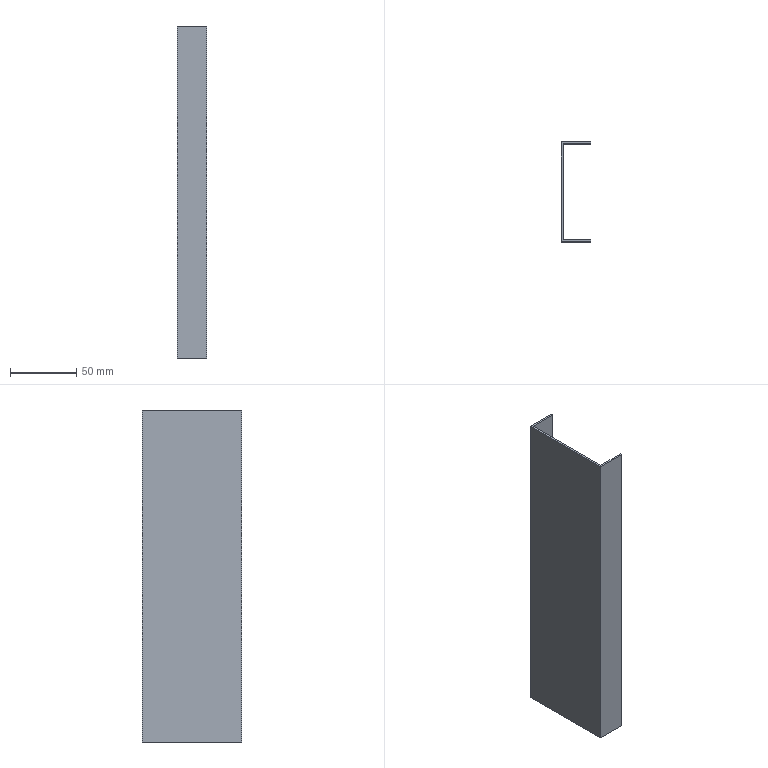Part | STEP file | Guide wheel mechanism revised.sldasm-Part-186 | 1 solid | 10 faces | box 22.5 x 75 x 250 mm | volume 43875 mm3 | plane 10
STEP:
#1=CARTESIAN_POINT('',(337.5,655.,202.));
#2=VERTEX_POINT('',#1);
#3=CARTESIAN_POINT('',(360.,655.,202.));
#4=VERTEX_POINT('',#3);
#5=CARTESIAN_POINT('',(337.5,655.,202.));
#6=DIRECTION('',(1.,0.,0.));
#7=VECTOR('',#6,1000.);
#8=LINE('',#5,#7);
#9=EDGE_CURVE('',#2,#4,#8,.T.);
#10=ORIENTED_EDGE('',*,*,#9,.F.);
#11=CARTESIAN_POINT('',(337.5,655.,-48.));
#12=VERTEX_POINT('',#11);
#13=CARTESIAN_POINT('',(337.5,655.,-48.));
#14=DIRECTION('',(0.,0.,1.));
#15=VECTOR('',#14,1000.);
#16=LINE('',#13,#15);
#17=EDGE_CURVE('',#12,#2,#16,.T.);
#18=ORIENTED_EDGE('',*,*,#17,.F.);
#19=CARTESIAN_POINT('',(360.,655.,-48.));
#20=VERTEX_POINT('',#19);
#21=CARTESIAN_POINT('',(337.5,655.,-48.));
#22=DIRECTION('',(1.,0.,0.));
#23=VECTOR('',#22,1000.);
#24=LINE('',#21,#23);
#25=EDGE_CURVE('',#12,#20,#24,.T.);
#26=ORIENTED_EDGE('',*,*,#25,.T.);
#27=CARTESIAN_POINT('',(360.,655.,-48.));
#28=DIRECTION('',(0.,0.,1.));
#29=VECTOR('',#28,1000.);
#30=LINE('',#27,#29);
#31=EDGE_CURVE('',#20,#4,#30,.T.);
#32=ORIENTED_EDGE('',*,*,#31,.T.);
#33=EDGE_LOOP('',(#10,#18,#26,#32));
#34=FACE_OUTER_BOUND('',#33,.T.);
#35=CARTESIAN_POINT('',(337.5,655.,-48.));
#36=DIRECTION('',(0.,-1.,0.));
#37=DIRECTION('',(0.,0.,-1.));
#38=AXIS2_PLACEMENT_3D('',#35,#36,#37);
#39=PLANE('',#38);
#40=ADVANCED_FACE('',(#34),#39,.T.);
#41=CARTESIAN_POINT('',(337.5,730.,202.));
#42=VERTEX_POINT('',#41);
#43=CARTESIAN_POINT('',(337.5,730.,202.));
#44=DIRECTION('',(0.,-1.,0.));
#45=VECTOR('',#44,1000.);
#46=LINE('',#43,#45);
#47=EDGE_CURVE('',#42,#2,#46,.T.);
#48=ORIENTED_EDGE('',*,*,#47,.F.);
#49=CARTESIAN_POINT('',(337.5,730.,-48.));
#50=VERTEX_POINT('',#49);
#51=CARTESIAN_POINT('',(337.5,730.,-48.));
#52=DIRECTION('',(0.,0.,1.));
#53=VECTOR('',#52,1000.);
#54=LINE('',#51,#53);
#55=EDGE_CURVE('',#50,#42,#54,.T.);
#56=ORIENTED_EDGE('',*,*,#55,.F.);
#57=CARTESIAN_POINT('',(337.5,730.,-48.));
#58=DIRECTION('',(0.,-1.,0.));
#59=VECTOR('',#58,1000.);
#60=LINE('',#57,#59);
#61=EDGE_CURVE('',#50,#12,#60,.T.);
#62=ORIENTED_EDGE('',*,*,#61,.T.);
#63=ORIENTED_EDGE('',*,*,#17,.T.);
#64=EDGE_LOOP('',(#48,#56,#62,#63));
#65=FACE_OUTER_BOUND('',#64,.T.);
#66=CARTESIAN_POINT('',(337.5,730.,-48.));
#67=DIRECTION('',(-1.,0.,0.));
#68=DIRECTION('',(0.,-1.,0.));
#69=AXIS2_PLACEMENT_3D('',#66,#67,#68);
#70=PLANE('',#69);
#71=ADVANCED_FACE('',(#65),#70,.T.);
#72=CARTESIAN_POINT('',(360.,730.,202.));
#73=VERTEX_POINT('',#72);
#74=CARTESIAN_POINT('',(337.5,730.,202.));
#75=DIRECTION('',(-1.,0.,0.));
#76=VECTOR('',#75,1000.);
#77=LINE('',#74,#76);
#78=EDGE_CURVE('',#73,#42,#77,.T.);
#79=ORIENTED_EDGE('',*,*,#78,.F.);
#80=CARTESIAN_POINT('',(360.,730.,-48.));
#81=VERTEX_POINT('',#80);
#82=CARTESIAN_POINT('',(360.,730.,-48.));
#83=DIRECTION('',(0.,0.,1.));
#84=VECTOR('',#83,1000.);
#85=LINE('',#82,#84);
#86=EDGE_CURVE('',#81,#73,#85,.T.);
#87=ORIENTED_EDGE('',*,*,#86,.F.);
#88=CARTESIAN_POINT('',(337.5,730.,-48.));
#89=DIRECTION('',(-1.,0.,0.));
#90=VECTOR('',#89,1000.);
#91=LINE('',#88,#90);
#92=EDGE_CURVE('',#81,#50,#91,.T.);
#93=ORIENTED_EDGE('',*,*,#92,.T.);
#94=ORIENTED_EDGE('',*,*,#55,.T.);
#95=EDGE_LOOP('',(#79,#87,#93,#94));
#96=FACE_OUTER_BOUND('',#95,.T.);
#97=CARTESIAN_POINT('',(337.5,730.,-48.));
#98=DIRECTION('',(0.,1.,0.));
#99=DIRECTION('',(0.,0.,1.));
#100=AXIS2_PLACEMENT_3D('',#97,#98,#99);
#101=PLANE('',#100);
#102=ADVANCED_FACE('',(#96),#101,.T.);
#103=CARTESIAN_POINT('',(360.,728.5,202.));
#104=VERTEX_POINT('',#103);
#105=CARTESIAN_POINT('',(360.,730.,202.));
#106=DIRECTION('',(0.,-1.,0.));
#107=VECTOR('',#106,1000.);
#108=LINE('',#105,#107);
#109=EDGE_CURVE('',#73,#104,#108,.T.);
#110=ORIENTED_EDGE('',*,*,#109,.T.);
#111=CARTESIAN_POINT('',(360.,728.5,-48.));
#112=VERTEX_POINT('',#111);
#113=CARTESIAN_POINT('',(360.,728.5,-48.));
#114=DIRECTION('',(0.,0.,1.));
#115=VECTOR('',#114,1000.);
#116=LINE('',#113,#115);
#117=EDGE_CURVE('',#112,#104,#116,.T.);
#118=ORIENTED_EDGE('',*,*,#117,.F.);
#119=CARTESIAN_POINT('',(360.,730.,-48.));
#120=DIRECTION('',(0.,-1.,0.));
#121=VECTOR('',#120,1000.);
#122=LINE('',#119,#121);
#123=EDGE_CURVE('',#81,#112,#122,.T.);
#124=ORIENTED_EDGE('',*,*,#123,.F.);
#125=ORIENTED_EDGE('',*,*,#86,.T.);
#126=EDGE_LOOP('',(#110,#118,#124,#125));
#127=FACE_OUTER_BOUND('',#126,.T.);
#128=CARTESIAN_POINT('',(360.,730.,-48.));
#129=DIRECTION('',(-1.,0.,0.));
#130=DIRECTION('',(0.,0.,1.));
#131=AXIS2_PLACEMENT_3D('',#128,#129,#130);
#132=PLANE('',#131);
#133=ADVANCED_FACE('',(#127),#132,.F.);
#134=CARTESIAN_POINT('',(339.,728.5,202.));
#135=VERTEX_POINT('',#134);
#136=CARTESIAN_POINT('',(337.5,728.5,202.));
#137=DIRECTION('',(-1.,0.,0.));
#138=VECTOR('',#137,1000.);
#139=LINE('',#136,#138);
#140=EDGE_CURVE('',#104,#135,#139,.T.);
#141=ORIENTED_EDGE('',*,*,#140,.T.);
#142=CARTESIAN_POINT('',(339.,728.5,-48.));
#143=VERTEX_POINT('',#142);
#144=CARTESIAN_POINT('',(339.,728.5,-48.));
#145=DIRECTION('',(0.,0.,1.));
#146=VECTOR('',#145,1000.);
#147=LINE('',#144,#146);
#148=EDGE_CURVE('',#143,#135,#147,.T.);
#149=ORIENTED_EDGE('',*,*,#148,.F.);
#150=CARTESIAN_POINT('',(337.5,728.5,-48.));
#151=DIRECTION('',(-1.,0.,0.));
#152=VECTOR('',#151,1000.);
#153=LINE('',#150,#152);
#154=EDGE_CURVE('',#112,#143,#153,.T.);
#155=ORIENTED_EDGE('',*,*,#154,.F.);
#156=ORIENTED_EDGE('',*,*,#117,.T.);
#157=EDGE_LOOP('',(#141,#149,#155,#156));
#158=FACE_OUTER_BOUND('',#157,.T.);
#159=CARTESIAN_POINT('',(337.5,728.5,-48.));
#160=DIRECTION('',(0.,1.,0.));
#161=DIRECTION('',(0.,0.,1.));
#162=AXIS2_PLACEMENT_3D('',#159,#160,#161);
#163=PLANE('',#162);
#164=ADVANCED_FACE('',(#158),#163,.F.);
#165=CARTESIAN_POINT('',(339.,656.5,202.));
#166=VERTEX_POINT('',#165);
#167=CARTESIAN_POINT('',(339.,730.,202.));
#168=DIRECTION('',(0.,-1.,0.));
#169=VECTOR('',#168,1000.);
#170=LINE('',#167,#169);
#171=EDGE_CURVE('',#135,#166,#170,.T.);
#172=ORIENTED_EDGE('',*,*,#171,.T.);
#173=CARTESIAN_POINT('',(339.,656.5,-48.));
#174=VERTEX_POINT('',#173);
#175=CARTESIAN_POINT('',(339.,656.5,-48.));
#176=DIRECTION('',(0.,0.,1.));
#177=VECTOR('',#176,1000.);
#178=LINE('',#175,#177);
#179=EDGE_CURVE('',#174,#166,#178,.T.);
#180=ORIENTED_EDGE('',*,*,#179,.F.);
#181=CARTESIAN_POINT('',(339.,730.,-48.));
#182=DIRECTION('',(0.,-1.,0.));
#183=VECTOR('',#182,1000.);
#184=LINE('',#181,#183);
#185=EDGE_CURVE('',#143,#174,#184,.T.);
#186=ORIENTED_EDGE('',*,*,#185,.F.);
#187=ORIENTED_EDGE('',*,*,#148,.T.);
#188=EDGE_LOOP('',(#172,#180,#186,#187));
#189=FACE_OUTER_BOUND('',#188,.T.);
#190=CARTESIAN_POINT('',(339.,730.,-48.));
#191=DIRECTION('',(-1.,0.,0.));
#192=DIRECTION('',(0.,-1.,0.));
#193=AXIS2_PLACEMENT_3D('',#190,#191,#192);
#194=PLANE('',#193);
#195=ADVANCED_FACE('',(#189),#194,.F.);
#196=CARTESIAN_POINT('',(360.,656.5,202.));
#197=VERTEX_POINT('',#196);
#198=CARTESIAN_POINT('',(337.5,656.5,202.));
#199=DIRECTION('',(1.,0.,0.));
#200=VECTOR('',#199,1000.);
#201=LINE('',#198,#200);
#202=EDGE_CURVE('',#166,#197,#201,.T.);
#203=ORIENTED_EDGE('',*,*,#202,.T.);
#204=CARTESIAN_POINT('',(360.,656.5,-48.));
#205=VERTEX_POINT('',#204);
#206=CARTESIAN_POINT('',(360.,656.5,-48.));
#207=DIRECTION('',(0.,0.,1.));
#208=VECTOR('',#207,1000.);
#209=LINE('',#206,#208);
#210=EDGE_CURVE('',#205,#197,#209,.T.);
#211=ORIENTED_EDGE('',*,*,#210,.F.);
#212=CARTESIAN_POINT('',(337.5,656.5,-48.));
#213=DIRECTION('',(1.,0.,0.));
#214=VECTOR('',#213,1000.);
#215=LINE('',#212,#214);
#216=EDGE_CURVE('',#174,#205,#215,.T.);
#217=ORIENTED_EDGE('',*,*,#216,.F.);
#218=ORIENTED_EDGE('',*,*,#179,.T.);
#219=EDGE_LOOP('',(#203,#211,#217,#218));
#220=FACE_OUTER_BOUND('',#219,.T.);
#221=CARTESIAN_POINT('',(337.5,656.5,-48.));
#222=DIRECTION('',(0.,-1.,0.));
#223=DIRECTION('',(0.,0.,-1.));
#224=AXIS2_PLACEMENT_3D('',#221,#222,#223);
#225=PLANE('',#224);
#226=ADVANCED_FACE('',(#220),#225,.F.);
#227=CARTESIAN_POINT('',(360.,656.5,202.));
#228=DIRECTION('',(0.,-1.,0.));
#229=VECTOR('',#228,1000.);
#230=LINE('',#227,#229);
#231=EDGE_CURVE('',#197,#4,#230,.T.);
#232=ORIENTED_EDGE('',*,*,#231,.T.);
#233=ORIENTED_EDGE('',*,*,#31,.F.);
#234=CARTESIAN_POINT('',(360.,656.5,-48.));
#235=DIRECTION('',(0.,-1.,0.));
#236=VECTOR('',#235,1000.);
#237=LINE('',#234,#236);
#238=EDGE_CURVE('',#205,#20,#237,.T.);
#239=ORIENTED_EDGE('',*,*,#238,.F.);
#240=ORIENTED_EDGE('',*,*,#210,.T.);
#241=EDGE_LOOP('',(#232,#233,#239,#240));
#242=FACE_OUTER_BOUND('',#241,.T.);
#243=CARTESIAN_POINT('',(360.,656.5,-48.));
#244=DIRECTION('',(-1.,0.,0.));
#245=DIRECTION('',(0.,0.,1.));
#246=AXIS2_PLACEMENT_3D('',#243,#244,#245);
#247=PLANE('',#246);
#248=ADVANCED_FACE('',(#242),#247,.F.);
#249=ORIENTED_EDGE('',*,*,#25,.F.);
#250=ORIENTED_EDGE('',*,*,#61,.F.);
#251=ORIENTED_EDGE('',*,*,#92,.F.);
#252=ORIENTED_EDGE('',*,*,#123,.T.);
#253=ORIENTED_EDGE('',*,*,#154,.T.);
#254=ORIENTED_EDGE('',*,*,#185,.T.);
#255=ORIENTED_EDGE('',*,*,#216,.T.);
#256=ORIENTED_EDGE('',*,*,#238,.T.);
#257=EDGE_LOOP('',(#249,#250,#251,#252,#253,#254,#255,#256));
#258=FACE_OUTER_BOUND('',#257,.T.);
#259=CARTESIAN_POINT('',(0.,0.,-48.));
#260=DIRECTION('',(0.,0.,-1.));
#261=DIRECTION('',(-1.,0.,0.));
#262=AXIS2_PLACEMENT_3D('',#259,#260,#261);
#263=PLANE('',#262);
#264=ADVANCED_FACE('',(#258),#263,.T.);
#265=ORIENTED_EDGE('',*,*,#9,.T.);
#266=ORIENTED_EDGE('',*,*,#231,.F.);
#267=ORIENTED_EDGE('',*,*,#202,.F.);
#268=ORIENTED_EDGE('',*,*,#171,.F.);
#269=ORIENTED_EDGE('',*,*,#140,.F.);
#270=ORIENTED_EDGE('',*,*,#109,.F.);
#271=ORIENTED_EDGE('',*,*,#78,.T.);
#272=ORIENTED_EDGE('',*,*,#47,.T.);
#273=EDGE_LOOP('',(#265,#266,#267,#268,#269,#270,#271,#272));
#274=FACE_OUTER_BOUND('',#273,.T.);
#275=CARTESIAN_POINT('',(0.,0.,202.));
#276=DIRECTION('',(0.,0.,-1.));
#277=DIRECTION('',(-1.,0.,0.));
#278=AXIS2_PLACEMENT_3D('',#275,#276,#277);
#279=PLANE('',#278);
#280=ADVANCED_FACE('',(#274),#279,.F.);
#281=CLOSED_SHELL('',(#40,#71,#102,#133,#164,#195,#226,#248,#264,#280));
#282=MANIFOLD_SOLID_BREP('',#281);
#283=CARTESIAN_POINT('',(0.,0.,0.));
#284=DIRECTION('',(0.,0.,1.));
#285=DIRECTION('',(1.,0.,0.));
#286=AXIS2_PLACEMENT_3D('',#283,#284,#285);
#287=(LENGTH_UNIT()NAMED_UNIT(*)SI_UNIT(.MILLI.,.METRE.));
#288=UNCERTAINTY_MEASURE_WITH_UNIT(LENGTH_MEASURE(0.00001),#287,'','');
#289=(NAMED_UNIT(*)PLANE_ANGLE_UNIT()SI_UNIT($,.RADIAN.));
#290=(NAMED_UNIT(*)SI_UNIT($,.STERADIAN.)SOLID_ANGLE_UNIT());
#291=(GEOMETRIC_REPRESENTATION_CONTEXT(3)GLOBAL_UNCERTAINTY_ASSIGNED_CONTEXT((#288))GLOBAL_UNIT_ASSIGNED_CONTEXT((#287,#289,#290))REPRESENTATION_CONTEXT('',''));
#292=ADVANCED_BREP_SHAPE_REPRESENTATION('',(#282,#286),#291);